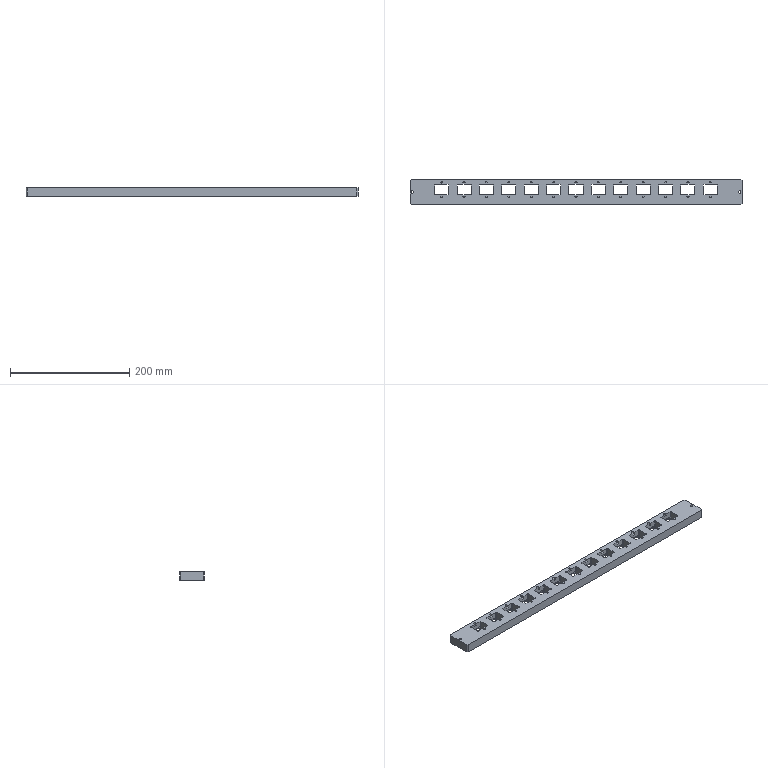NC program | NX | posted with a generic post | part box 556 x 41 x 15 mm
Lines 1 to 872 of 52182:
N10 G17 G21 G94 G90
(ZLEVEL_PROFILE_COPY_1_COPY_COPY_3 , TOOL : D6JING)
N12 T06 M6
N14 G54
N16 G17 G0 G90 X220.712 Y-3.45 S5000 M3
N18 G43 Z30. H6
N20 Z-0.147
N22 G94 G1 X219.631 Y-4.121 F1000.
N24 G3 X219.348 Y-4.65 R0.6
N26 G1 X230.652 F1800.
N28 G3 X230.369 Y-4.121 R0.6
N30 G1 X229.288 Y-3.45
N32 G0 X220.712 Z-0.294
N34 G1 X219.631 Y-4.121 F1000.
N36 G3 X219.348 Y-4.65 R0.6
N38 G1 X230.652 F1800.
N40 G3 X230.369 Y-4.121 R0.6
N42 G1 X229.288 Y-3.45
N44 G0 X220.712 Z-0.441
N46 G1 X219.631 Y-4.121 F1000.
N48 G3 X219.348 Y-4.65 R0.6
N50 G1 X230.652 F1800.
N52 G3 X230.369 Y-4.121 R0.6
N54 G1 X229.288 Y-3.45
N56 G0 X220.712 Z-0.588
N58 G1 X219.631 Y-4.121 F1000.
N60 G3 X219.348 Y-4.65 R0.6
N62 G1 X230.652 F1800.
N64 G3 X230.369 Y-4.121 R0.6
N66 G1 X229.288 Y-3.45
N68 G0 X220.712 Z-0.735
N70 G1 X219.631 Y-4.121 F1000.
N72 G3 X219.348 Y-4.65 R0.6
N74 G1 X230.652 F1800.
N76 G3 X230.369 Y-4.121 R0.6
N78 G1 X229.288 Y-3.45
N80 G0 X220.712 Z-0.882
N82 G1 X219.631 Y-4.121 F1000.
N84 G3 X219.348 Y-4.65 R0.6
N86 G1 X230.652 F1800.
N88 G3 X230.369 Y-4.121 R0.6
N90 G1 X229.288 Y-3.45
N92 G0 X220.712 Z-1.029
N94 G1 X219.631 Y-4.121 F1000.
N96 G3 X219.348 Y-4.65 R0.6
N98 G1 X230.652 F1800.
N100 G3 X230.369 Y-4.121 R0.6
N102 G1 X229.288 Y-3.45
N104 G0 X220.712 Z-1.176
N106 G1 X219.631 Y-4.121 F1000.
N108 G3 X219.348 Y-4.65 R0.6
N110 G1 X230.652 F1800.
N112 G3 X230.369 Y-4.121 R0.6
N114 G1 X229.288 Y-3.45
N116 G0 X220.712 Z-1.324
N118 G1 X219.631 Y-4.121 F1000.
N120 G3 X219.348 Y-4.65 R0.6
N122 G1 X230.652 F1800.
N124 G3 X230.369 Y-4.121 R0.6
N126 G1 X229.288 Y-3.45
N128 G0 X220.712 Z-1.471
N130 G1 X219.631 Y-4.121 F1000.
N132 G3 X219.348 Y-4.65 R0.6
N134 G1 X230.652 F1800.
N136 G3 X230.369 Y-4.121 R0.6
N138 G1 X229.288 Y-3.45
N140 G0 X220.712 Z-1.618
N142 G1 X219.631 Y-4.121 F1000.
N144 G3 X219.348 Y-4.65 R0.6
N146 G1 X230.652 F1800.
N148 G3 X230.369 Y-4.121 R0.6
N150 G1 X229.288 Y-3.45
N152 G0 X220.712 Z-1.765
N154 G1 X219.631 Y-4.121 F1000.
N156 G3 X219.348 Y-4.65 R0.6
N158 G1 X230.652 F1800.
N160 G3 X230.369 Y-4.121 R0.6
N162 G1 X229.288 Y-3.45
N164 G0 X220.712 Z-1.912
N166 G1 X219.631 Y-4.121 F1000.
N168 G3 X219.348 Y-4.65 R0.6
N170 G1 X230.652 F1800.
N172 G3 X230.369 Y-4.121 R0.6
N174 G1 X229.288 Y-3.45
N176 G0 X220.712 Z-2.059
N178 G1 X219.631 Y-4.121 F1000.
N180 G3 X219.348 Y-4.65 R0.6
N182 G1 X230.652 F1800.
N184 G3 X230.369 Y-4.121 R0.6
N186 G1 X229.288 Y-3.45
N188 G0 X220.712 Z-2.206
N190 G1 X219.631 Y-4.121 F1000.
N192 G3 X219.348 Y-4.65 R0.6
N194 G1 X230.652 F1800.
N196 G3 X230.369 Y-4.121 R0.6
N198 G1 X229.288 Y-3.45
N200 G0 X220.712 Z-2.353
N202 G1 X219.631 Y-4.121 F1000.
N204 G3 X219.348 Y-4.65 R0.6
N206 G1 X230.652 F1800.
N208 G3 X230.369 Y-4.121 R0.6
N210 G1 X229.288 Y-3.45
N212 G0 X220.712 Z-2.5
N214 G1 X219.631 Y-4.121 F1000.
N216 G3 X219.348 Y-4.65 R0.6
N218 G1 X230.652 F1800.
N220 G3 X230.369 Y-4.121 R0.6
N222 G1 X229.288 Y-3.45
N224 G0 X220.712 Z-2.647
N226 G1 X219.631 Y-4.121 F1000.
N228 G3 X219.348 Y-4.65 R0.6
N230 G1 X230.652 F1800.
N232 G3 X230.369 Y-4.121 R0.6
N234 G1 X229.288 Y-3.45
N236 G0 X220.712 Z-2.794
N238 G1 X219.631 Y-4.121 F1000.
N240 G3 X219.348 Y-4.65 R0.6
N242 G1 X230.652 F1800.
N244 G3 X230.369 Y-4.121 R0.6
N246 G1 X229.288 Y-3.45
N248 G0 X220.712 Z-2.941
N250 G1 X219.631 Y-4.121 F1000.
N252 G3 X219.348 Y-4.65 R0.6
N254 G1 X230.652 F1800.
N256 G3 X230.369 Y-4.121 R0.6
N258 G1 X229.288 Y-3.45
N260 G0 X220.712 Z-3.088
N262 G1 X219.631 Y-4.121 F1000.
N264 G3 X219.348 Y-4.65 R0.6
N266 G1 X230.652 F1800.
N268 G3 X230.369 Y-4.121 R0.6
N270 G1 X229.288 Y-3.45
N272 G0 X220.712 Z-3.235
N274 G1 X219.631 Y-4.121 F1000.
N276 G3 X219.348 Y-4.65 R0.6
N278 G1 X230.652 F1800.
N280 G3 X230.369 Y-4.121 R0.6
N282 G1 X229.288 Y-3.45
N284 G0 X220.712 Z-3.382
N286 G1 X219.631 Y-4.121 F1000.
N288 G3 X219.348 Y-4.65 R0.6
N290 G1 X230.652 F1800.
N292 G3 X230.369 Y-4.121 R0.6
N294 G1 X229.288 Y-3.45
N296 G0 X220.712 Z-3.529
N298 G1 X219.631 Y-4.121 F1000.
N300 G3 X219.348 Y-4.65 R0.6
N302 G1 X230.652 F1800.
N304 G3 X230.369 Y-4.121 R0.6
N306 G1 X229.288 Y-3.45
N308 G0 X220.712 Z-3.676
N310 G1 X219.631 Y-4.121 F1000.
N312 G3 X219.348 Y-4.65 R0.6
N314 G1 X230.652 F1800.
N316 G3 X230.369 Y-4.121 R0.6
N318 G1 X229.288 Y-3.45
N320 G0 X220.712 Z-3.824
N322 G1 X219.631 Y-4.121 F1000.
N324 G3 X219.348 Y-4.65 R0.6
N326 G1 X230.652 F1800.
N328 G3 X230.369 Y-4.121 R0.6
N330 G1 X229.288 Y-3.45
N332 G0 X220.712 Z-3.971
N334 G1 X219.631 Y-4.121 F1000.
N336 G3 X219.348 Y-4.65 R0.6
N338 G1 X230.652 F1800.
N340 G3 X230.369 Y-4.121 R0.6
N342 G1 X229.288 Y-3.45
N344 G0 X220.712 Z-4.118
N346 G1 X219.631 Y-4.121 F1000.
N348 G3 X219.348 Y-4.65 R0.6
N350 G1 X230.652 F1800.
N352 G3 X230.369 Y-4.121 R0.6
N354 G1 X229.288 Y-3.45
N356 G0 X220.712 Z-4.265
N358 G1 X219.631 Y-4.121 F1000.
N360 G3 X219.348 Y-4.65 R0.6
N362 G1 X230.652 F1800.
N364 G3 X230.369 Y-4.121 R0.6
N366 G1 X229.288 Y-3.45
N368 G0 X220.712 Z-4.412
N370 G1 X219.631 Y-4.121 F1000.
N372 G3 X219.348 Y-4.65 R0.6
N374 G1 X230.652 F1800.
N376 G3 X230.369 Y-4.121 R0.6
N378 G1 X229.288 Y-3.45
N380 G0 X220.712 Z-4.559
N382 G1 X219.631 Y-4.121 F1000.
N384 G3 X219.348 Y-4.65 R0.6
N386 G1 X230.652 F1800.
N388 G3 X230.369 Y-4.121 R0.6
N390 G1 X229.288 Y-3.45
N392 G0 X220.712 Z-4.706
N394 G1 X219.631 Y-4.121 F1000.
N396 G3 X219.348 Y-4.65 R0.6
N398 G1 X230.652 F1800.
N400 G3 X230.369 Y-4.121 R0.6
N402 G1 X229.288 Y-3.45
N404 G0 X220.712 Z-4.853
N406 G1 X219.631 Y-4.121 F1000.
N408 G3 X219.348 Y-4.65 R0.6
N410 G1 X230.652 F1800.
N412 G3 X230.369 Y-4.121 R0.6
N414 G1 X229.288 Y-3.45
N416 G0 X220.712 Z-5.
N418 G1 X219.631 Y-4.121 F1000.
N420 G3 X219.348 Y-4.65 R0.6
N422 G1 X230.652 F1800.
N424 G3 X230.369 Y-4.121 R0.6
N426 G1 X229.288 Y-3.45
N428 G0 Z30.
N430 Y11.45
N432 Z-0.147
N434 G1 X230.369 Y12.121 F1000.
N436 G3 X230.652 Y12.65 R0.6
N438 G1 X219.348 F1800.
N440 G3 X219.631 Y12.121 R0.6
N442 G1 X220.712 Y11.45
N444 G0 X229.288 Z-0.294
N446 G1 X230.369 Y12.121 F1000.
N448 G3 X230.652 Y12.65 R0.6
N450 G1 X219.348 F1800.
N452 G3 X219.631 Y12.121 R0.6
N454 G1 X220.712 Y11.45
N456 G0 X229.288 Z-0.441
N458 G1 X230.369 Y12.121 F1000.
N460 G3 X230.652 Y12.65 R0.6
N462 G1 X219.348 F1800.
N464 G3 X219.631 Y12.121 R0.6
N466 G1 X220.712 Y11.45
N468 G0 X229.288 Z-0.588
N470 G1 X230.369 Y12.121 F1000.
N472 G3 X230.652 Y12.65 R0.6
N474 G1 X219.348 F1800.
N476 G3 X219.631 Y12.121 R0.6
N478 G1 X220.712 Y11.45
N480 G0 X229.288 Z-0.735
N482 G1 X230.369 Y12.121 F1000.
N484 G3 X230.652 Y12.65 R0.6
N486 G1 X219.348 F1800.
N488 G3 X219.631 Y12.121 R0.6
N490 G1 X220.712 Y11.45
N492 G0 X229.288 Z-0.882
N494 G1 X230.369 Y12.121 F1000.
N496 G3 X230.652 Y12.65 R0.6
N498 G1 X219.348 F1800.
N500 G3 X219.631 Y12.121 R0.6
N502 G1 X220.712 Y11.45
N504 G0 X229.288 Z-1.029
N506 G1 X230.369 Y12.121 F1000.
N508 G3 X230.652 Y12.65 R0.6
N510 G1 X219.348 F1800.
N512 G3 X219.631 Y12.121 R0.6
N514 G1 X220.712 Y11.45
N516 G0 X229.288 Z-1.176
N518 G1 X230.369 Y12.121 F1000.
N520 G3 X230.652 Y12.65 R0.6
N522 G1 X219.348 F1800.
N524 G3 X219.631 Y12.121 R0.6
N526 G1 X220.712 Y11.45
N528 G0 X229.288 Z-1.324
N530 G1 X230.369 Y12.121 F1000.
N532 G3 X230.652 Y12.65 R0.6
N534 G1 X219.348 F1800.
N536 G3 X219.631 Y12.121 R0.6
N538 G1 X220.712 Y11.45
N540 G0 X229.288 Z-1.471
N542 G1 X230.369 Y12.121 F1000.
N544 G3 X230.652 Y12.65 R0.6
N546 G1 X219.348 F1800.
N548 G3 X219.631 Y12.121 R0.6
N550 G1 X220.712 Y11.45
N552 G0 X229.288 Z-1.618
N554 G1 X230.369 Y12.121 F1000.
N556 G3 X230.652 Y12.65 R0.6
N558 G1 X219.348 F1800.
N560 G3 X219.631 Y12.121 R0.6
N562 G1 X220.712 Y11.45
N564 G0 X229.288 Z-1.765
N566 G1 X230.369 Y12.121 F1000.
N568 G3 X230.652 Y12.65 R0.6
N570 G1 X219.348 F1800.
N572 G3 X219.631 Y12.121 R0.6
N574 G1 X220.712 Y11.45
N576 G0 X229.288 Z-1.912
N578 G1 X230.369 Y12.121 F1000.
N580 G3 X230.652 Y12.65 R0.6
N582 G1 X219.348 F1800.
N584 G3 X219.631 Y12.121 R0.6
N586 G1 X220.712 Y11.45
N588 G0 X229.288 Z-2.059
N590 G1 X230.369 Y12.121 F1000.
N592 G3 X230.652 Y12.65 R0.6
N594 G1 X219.348 F1800.
N596 G3 X219.631 Y12.121 R0.6
N598 G1 X220.712 Y11.45
N600 G0 X229.288 Z-2.206
N602 G1 X230.369 Y12.121 F1000.
N604 G3 X230.652 Y12.65 R0.6
N606 G1 X219.348 F1800.
N608 G3 X219.631 Y12.121 R0.6
N610 G1 X220.712 Y11.45
N612 G0 X229.288 Z-2.353
N614 G1 X230.369 Y12.121 F1000.
N616 G3 X230.652 Y12.65 R0.6
N618 G1 X219.348 F1800.
N620 G3 X219.631 Y12.121 R0.6
N622 G1 X220.712 Y11.45
N624 G0 X229.288 Z-2.5
N626 G1 X230.369 Y12.121 F1000.
N628 G3 X230.652 Y12.65 R0.6
N630 G1 X219.348 F1800.
N632 G3 X219.631 Y12.121 R0.6
N634 G1 X220.712 Y11.45
N636 G0 X229.288 Z-2.647
N638 G1 X230.369 Y12.121 F1000.
N640 G3 X230.652 Y12.65 R0.6
N642 G1 X219.348 F1800.
N644 G3 X219.631 Y12.121 R0.6
N646 G1 X220.712 Y11.45
N648 G0 X229.288 Z-2.794
N650 G1 X230.369 Y12.121 F1000.
N652 G3 X230.652 Y12.65 R0.6
N654 G1 X219.348 F1800.
N656 G3 X219.631 Y12.121 R0.6
N658 G1 X220.712 Y11.45
N660 G0 X229.288 Z-2.941
N662 G1 X230.369 Y12.121 F1000.
N664 G3 X230.652 Y12.65 R0.6
N666 G1 X219.348 F1800.
N668 G3 X219.631 Y12.121 R0.6
N670 G1 X220.712 Y11.45
N672 G0 X229.288 Z-3.088
N674 G1 X230.369 Y12.121 F1000.
N676 G3 X230.652 Y12.65 R0.6
N678 G1 X219.348 F1800.
N680 G3 X219.631 Y12.121 R0.6
N682 G1 X220.712 Y11.45
N684 G0 X229.288 Z-3.235
N686 G1 X230.369 Y12.121 F1000.
N688 G3 X230.652 Y12.65 R0.6
N690 G1 X219.348 F1800.
N692 G3 X219.631 Y12.121 R0.6
N694 G1 X220.712 Y11.45
N696 G0 X229.288 Z-3.382
N698 G1 X230.369 Y12.121 F1000.
N700 G3 X230.652 Y12.65 R0.6
N702 G1 X219.348 F1800.
N704 G3 X219.631 Y12.121 R0.6
N706 G1 X220.712 Y11.45
N708 G0 X229.288 Z-3.529
N710 G1 X230.369 Y12.121 F1000.
N712 G3 X230.652 Y12.65 R0.6
N714 G1 X219.348 F1800.
N716 G3 X219.631 Y12.121 R0.6
N718 G1 X220.712 Y11.45
N720 G0 X229.288 Z-3.676
N722 G1 X230.369 Y12.121 F1000.
N724 G3 X230.652 Y12.65 R0.6
N726 G1 X219.348 F1800.
N728 G3 X219.631 Y12.121 R0.6
N730 G1 X220.712 Y11.45
N732 G0 X229.288 Z-3.824
N734 G1 X230.369 Y12.121 F1000.
N736 G3 X230.652 Y12.65 R0.6
N738 G1 X219.348 F1800.
N740 G3 X219.631 Y12.121 R0.6
N742 G1 X220.712 Y11.45
N744 G0 X229.288 Z-3.971
N746 G1 X230.369 Y12.121 F1000.
N748 G3 X230.652 Y12.65 R0.6
N750 G1 X219.348 F1800.
N752 G3 X219.631 Y12.121 R0.6
N754 G1 X220.712 Y11.45
N756 G0 X229.288 Z-4.118
N758 G1 X230.369 Y12.121 F1000.
N760 G3 X230.652 Y12.65 R0.6
N762 G1 X219.348 F1800.
N764 G3 X219.631 Y12.121 R0.6
N766 G1 X220.712 Y11.45
N768 G0 X229.288 Z-4.265
N770 G1 X230.369 Y12.121 F1000.
N772 G3 X230.652 Y12.65 R0.6
N774 G1 X219.348 F1800.
N776 G3 X219.631 Y12.121 R0.6
N778 G1 X220.712 Y11.45
N780 G0 X229.288 Z-4.412
N782 G1 X230.369 Y12.121 F1000.
N784 G3 X230.652 Y12.65 R0.6
N786 G1 X219.348 F1800.
N788 G3 X219.631 Y12.121 R0.6
N790 G1 X220.712 Y11.45
N792 G0 X229.288 Z-4.559
N794 G1 X230.369 Y12.121 F1000.
N796 G3 X230.652 Y12.65 R0.6
N798 G1 X219.348 F1800.
N800 G3 X219.631 Y12.121 R0.6
N802 G1 X220.712 Y11.45
N804 G0 X229.288 Z-4.706
N806 G1 X230.369 Y12.121 F1000.
N808 G3 X230.652 Y12.65 R0.6
N810 G1 X219.348 F1800.
N812 G3 X219.631 Y12.121 R0.6
N814 G1 X220.712 Y11.45
N816 G0 X229.288 Z-4.853
N818 G1 X230.369 Y12.121 F1000.
N820 G3 X230.652 Y12.65 R0.6
N822 G1 X219.348 F1800.
N824 G3 X219.631 Y12.121 R0.6
N826 G1 X220.712 Y11.45
N828 G0 X229.288 Z-5.
N830 G1 X230.369 Y12.121 F1000.
N832 G3 X230.652 Y12.65 R0.6
N834 G1 X219.348 F1800.
N836 G3 X219.631 Y12.121 R0.6
N838 G1 X220.712 Y11.45
N840 G0 Z30.
N842 X183.212 Y-3.45
N844 Z-0.147
N846 G1 X182.131 Y-4.121 F1000.
N848 G3 X181.848 Y-4.65 R0.6
N850 G1 X193.152 F1800.
N852 G3 X192.869 Y-4.121 R0.6
N854 G1 X191.788 Y-3.45
N856 G0 X183.212 Z-0.294
N858 G1 X182.131 Y-4.121 F1000.
N860 G3 X181.848 Y-4.65 R0.6
N862 G1 X193.152 F1800.
N864 G3 X192.869 Y-4.121 R0.6
N866 G1 X191.788 Y-3.45
N868 G0 X183.212 Z-0.441
N870 G1 X182.131 Y-4.121 F1000.
N872 G3 X181.848 Y-4.65 R0.6
N874 G1 X193.152 F1800.
N876 G3 X192.869 Y-4.121 R0.6
N878 G1 X191.788 Y-3.45
N880 G0 X183.212 Z-0.588
N882 G1 X182.131 Y-4.121 F1000.
N884 G3 X181.848 Y-4.65 R0.6
N886 G1 X193.152 F1800.
N888 G3 X192.869 Y-4.121 R0.6
N890 G1 X191.788 Y-3.45
N892 G0 X183.212 Z-0.735
N894 G1 X182.131 Y-4.121 F1000.
N896 G3 X181.848 Y-4.65 R0.6
N898 G1 X193.152 F1800.
N900 G3 X192.869 Y-4.121 R0.6
N902 G1 X191.788 Y-3.45
N904 G0 X183.212 Z-0.882
N906 G1 X182.131 Y-4.121 F1000.
N908 G3 X181.848 Y-4.65 R0.6
N910 G1 X193.152 F1800.
N912 G3 X192.869 Y-4.121 R0.6
N914 G1 X191.788 Y-3.45
N916 G0 X183.212 Z-1.029
N918 G1 X182.131 Y-4.121 F1000.
N920 G3 X181.848 Y-4.65 R0.6
N922 G1 X193.152 F1800.
N924 G3 X192.869 Y-4.121 R0.6
N926 G1 X191.788 Y-3.45
N928 G0 X183.212 Z-1.176
N930 G1 X182.131 Y-4.121 F1000.
N932 G3 X181.848 Y-4.65 R0.6
N934 G1 X193.152 F1800.
N936 G3 X192.869 Y-4.121 R0.6
N938 G1 X191.788 Y-3.45
N940 G0 X183.212 Z-1.324
N942 G1 X182.131 Y-4.121 F1000.
N944 G3 X181.848 Y-4.65 R0.6
N946 G1 X193.152 F1800.
N948 G3 X192.869 Y-4.121 R0.6
N950 G1 X191.788 Y-3.45
N952 G0 X183.212 Z-1.471
N954 G1 X182.131 Y-4.121 F1000.
N956 G3 X181.848 Y-4.65 R0.6
N958 G1 X193.152 F1800.
N960 G3 X192.869 Y-4.121 R0.6
N962 G1 X191.788 Y-3.45
N964 G0 X183.212 Z-1.618
N966 G1 X182.131 Y-4.121 F1000.
N968 G3 X181.848 Y-4.65 R0.6
N970 G1 X193.152 F1800.
N972 G3 X192.869 Y-4.121 R0.6
N974 G1 X191.788 Y-3.45
N976 G0 X183.212 Z-1.765
N978 G1 X182.131 Y-4.121 F1000.
N980 G3 X181.848 Y-4.65 R0.6
N982 G1 X193.152 F1800.
N984 G3 X192.869 Y-4.121 R0.6
N986 G1 X191.788 Y-3.45
N988 G0 X183.212 Z-1.912
N990 G1 X182.131 Y-4.121 F1000.
N992 G3 X181.848 Y-4.65 R0.6
N994 G1 X193.152 F1800.
N996 G3 X192.869 Y-4.121 R0.6
N998 G1 X191.788 Y-3.45
N1000 G0 X183.212 Z-2.059
N1002 G1 X182.131 Y-4.121 F1000.
N1004 G3 X181.848 Y-4.65 R0.6
N1006 G1 X193.152 F1800.
N1008 G3 X192.869 Y-4.121 R0.6
N1010 G1 X191.788 Y-3.45
N1012 G0 X183.212 Z-2.206
N1014 G1 X182.131 Y-4.121 F1000.
N1016 G3 X181.848 Y-4.65 R0.6
N1018 G1 X193.152 F1800.
N1020 G3 X192.869 Y-4.121 R0.6
N1022 G1 X191.788 Y-3.45
N1024 G0 X183.212 Z-2.353
N1026 G1 X182.131 Y-4.121 F1000.
N1028 G3 X181.848 Y-4.65 R0.6
N1030 G1 X193.152 F1800.
N1032 G3 X192.869 Y-4.121 R0.6
N1034 G1 X191.788 Y-3.45
N1036 G0 X183.212 Z-2.5
N1038 G1 X182.131 Y-4.121 F1000.
N1040 G3 X181.848 Y-4.65 R0.6
N1042 G1 X193.152 F1800.
N1044 G3 X192.869 Y-4.121 R0.6
N1046 G1 X191.788 Y-3.45
N1048 G0 X183.212 Z-2.647
N1050 G1 X182.131 Y-4.121 F1000.
N1052 G3 X181.848 Y-4.65 R0.6
N1054 G1 X193.152 F1800.
N1056 G3 X192.869 Y-4.121 R0.6
N1058 G1 X191.788 Y-3.45
N1060 G0 X183.212 Z-2.794
N1062 G1 X182.131 Y-4.121 F1000.
N1064 G3 X181.848 Y-4.65 R0.6
N1066 G1 X193.152 F1800.
N1068 G3 X192.869 Y-4.121 R0.6
N1070 G1 X191.788 Y-3.45
N1072 G0 X183.212 Z-2.941
N1074 G1 X182.131 Y-4.121 F1000.
N1076 G3 X181.848 Y-4.65 R0.6
N1078 G1 X193.152 F1800.
N1080 G3 X192.869 Y-4.121 R0.6
N1082 G1 X191.788 Y-3.45
N1084 G0 X183.212 Z-3.088
N1086 G1 X182.131 Y-4.121 F1000.
N1088 G3 X181.848 Y-4.65 R0.6
N1090 G1 X193.152 F1800.
N1092 G3 X192.869 Y-4.121 R0.6
N1094 G1 X191.788 Y-3.45
N1096 G0 X183.212 Z-3.235
N1098 G1 X182.131 Y-4.121 F1000.
N1100 G3 X181.848 Y-4.65 R0.6
N1102 G1 X193.152 F1800.
N1104 G3 X192.869 Y-4.121 R0.6
N1106 G1 X191.788 Y-3.45
N1108 G0 X183.212 Z-3.382
N1110 G1 X182.131 Y-4.121 F1000.
N1112 G3 X181.848 Y-4.65 R0.6
N1114 G1 X193.152 F1800.
N1116 G3 X192.869 Y-4.121 R0.6
N1118 G1 X191.788 Y-3.45
N1120 G0 X183.212 Z-3.529
N1122 G1 X182.131 Y-4.121 F1000.
N1124 G3 X181.848 Y-4.65 R0.6
N1126 G1 X193.152 F1800.
N1128 G3 X192.869 Y-4.121 R0.6
N1130 G1 X191.788 Y-3.45
N1132 G0 X183.212 Z-3.676
N1134 G1 X182.131 Y-4.121 F1000.
N1136 G3 X181.848 Y-4.65 R0.6
N1138 G1 X193.152 F1800.
N1140 G3 X192.869 Y-4.121 R0.6
N1142 G1 X191.788 Y-3.45
N1144 G0 X183.212 Z-3.824
N1146 G1 X182.131 Y-4.121 F1000.
N1148 G3 X181.848 Y-4.65 R0.6
N1150 G1 X193.152 F1800.
N1152 G3 X192.869 Y-4.121 R0.6
N1154 G1 X191.788 Y-3.45
N1156 G0 X183.212 Z-3.971
N1158 G1 X182.131 Y-4.121 F1000.
N1160 G3 X181.848 Y-4.65 R0.6
N1162 G1 X193.152 F1800.
N1164 G3 X192.869 Y-4.121 R0.6
N1166 G1 X191.788 Y-3.45
N1168 G0 X183.212 Z-4.118
N1170 G1 X182.131 Y-4.121 F1000.
N1172 G3 X181.848 Y-4.65 R0.6
N1174 G1 X193.152 F1800.
N1176 G3 X192.869 Y-4.121 R0.6
N1178 G1 X191.788 Y-3.45
N1180 G0 X183.212 Z-4.265
N1182 G1 X182.131 Y-4.121 F1000.
N1184 G3 X181.848 Y-4.65 R0.6
N1186 G1 X193.152 F1800.
N1188 G3 X192.869 Y-4.121 R0.6
N1190 G1 X191.788 Y-3.45
N1192 G0 X183.212 Z-4.412
N1194 G1 X182.131 Y-4.121 F1000.
N1196 G3 X181.848 Y-4.65 R0.6
N1198 G1 X193.152 F1800.
N1200 G3 X192.869 Y-4.121 R0.6
N1202 G1 X191.788 Y-3.45
N1204 G0 X183.212 Z-4.559
N1206 G1 X182.131 Y-4.121 F1000.
N1208 G3 X181.848 Y-4.65 R0.6
N1210 G1 X193.152 F1800.
N1212 G3 X192.869 Y-4.121 R0.6
N1214 G1 X191.788 Y-3.45
N1216 G0 X183.212 Z-4.706
N1218 G1 X182.131 Y-4.121 F1000.
N1220 G3 X181.848 Y-4.65 R0.6
N1222 G1 X193.152 F1800.
N1224 G3 X192.869 Y-4.121 R0.6
N1226 G1 X191.788 Y-3.45
N1228 G0 X183.212 Z-4.853
N1230 G1 X182.131 Y-4.121 F1000.
N1232 G3 X181.848 Y-4.65 R0.6
N1234 G1 X193.152 F1800.
N1236 G3 X192.869 Y-4.121 R0.6
N1238 G1 X191.788 Y-3.45
N1240 G0 X183.212 Z-5.
N1242 G1 X182.131 Y-4.121 F1000.
N1244 G3 X181.848 Y-4.65 R0.6
N1246 G1 X193.152 F1800.
N1248 G3 X192.869 Y-4.121 R0.6
N1250 G1 X191.788 Y-3.45
N1252 G0 Z30.
N1254 Y11.45
N1256 Z-0.147
N1258 G1 X192.869 Y12.121 F1000.
N1260 G3 X193.152 Y12.65 R0.6
N1262 G1 X181.848 F1800.
N1264 G3 X182.131 Y12.121 R0.6
N1266 G1 X183.212 Y11.45
N1268 G0 X191.788 Z-0.294
N1270 G1 X192.869 Y12.121 F1000.
N1272 G3 X193.152 Y12.65 R0.6
N1274 G1 X181.848 F1800.
N1276 G3 X182.131 Y12.121 R0.6
N1278 G1 X183.212 Y11.45
N1280 G0 X191.788 Z-0.441
N1282 G1 X192.869 Y12.121 F1000.
N1284 G3 X193.152 Y12.65 R0.6
N1286 G1 X181.848 F1800.
N1288 G3 X182.131 Y12.121 R0.6
N1290 G1 X183.212 Y11.45
N1292 G0 X191.788 Z-0.588
N1294 G1 X192.869 Y12.121 F1000.
N1296 G3 X193.152 Y12.65 R0.6
N1298 G1 X181.848 F1800.
N1300 G3 X182.131 Y12.121 R0.6
N1302 G1 X183.212 Y11.45
N1304 G0 X191.788 Z-0.735
N1306 G1 X192.869 Y12.121 F1000.
N1308 G3 X193.152 Y12.65 R0.6
N1310 G1 X181.848 F1800.
N1312 G3 X182.131 Y12.121 R0.6
N1314 G1 X183.212 Y11.45
N1316 G0 X191.788 Z-0.882
N1318 G1 X192.869 Y12.121 F1000.
N1320 G3 X193.152 Y12.65 R0.6
N1322 G1 X181.848 F1800.
N1324 G3 X182.131 Y12.121 R0.6
N1326 G1 X183.212 Y11.45
N1328 G0 X191.788 Z-1.029
N1330 G1 X192.869 Y12.121 F1000.
N1332 G3 X193.152 Y12.65 R0.6
N1334 G1 X181.848 F1800.
N1336 G3 X182.131 Y12.121 R0.6
N1338 G1 X183.212 Y11.45
N1340 G0 X191.788 Z-1.176
N1342 G1 X192.869 Y12.121 F1000.
N1344 G3 X193.152 Y12.65 R0.6
N1346 G1 X181.848 F1800.
N1348 G3 X182.131 Y12.121 R0.6
N1350 G1 X183.212 Y11.45
N1352 G0 X191.788 Z-1.324
N1354 G1 X192.869 Y12.121 F1000.
N1356 G3 X193.152 Y12.65 R0.6
N1358 G1 X181.848 F1800.
N1360 G3 X182.131 Y12.121 R0.6
N1362 G1 X183.212 Y11.45
N1364 G0 X191.788 Z-1.471
N1366 G1 X192.869 Y12.121 F1000.
N1368 G3 X193.152 Y12.65 R0.6
N1370 G1 X181.848 F1800.
N1372 G3 X182.131 Y12.121 R0.6
N1374 G1 X183.212 Y11.45
N1376 G0 X191.788 Z-1.618
N1378 G1 X192.869 Y12.121 F1000.
N1380 G3 X193.152 Y12.65 R0.6
N1382 G1 X181.848 F1800.
N1384 G3 X182.131 Y12.121 R0.6
N1386 G1 X183.212 Y11.45
N1388 G0 X191.788 Z-1.765
N1390 G1 X192.869 Y12.121 F1000.
N1392 G3 X193.152 Y12.65 R0.6
N1394 G1 X181.848 F1800.
N1396 G3 X182.131 Y12.121 R0.6
N1398 G1 X183.212 Y11.45
N1400 G0 X191.788 Z-1.912
N1402 G1 X192.869 Y12.121 F1000.
N1404 G3 X193.152 Y12.65 R0.6
N1406 G1 X181.848 F1800.
N1408 G3 X182.131 Y12.121 R0.6
N1410 G1 X183.212 Y11.45
N1412 G0 X191.788 Z-2.059
N1414 G1 X192.869 Y12.121 F1000.
N1416 G3 X193.152 Y12.65 R0.6
N1418 G1 X181.848 F1800.
N1420 G3 X182.131 Y12.121 R0.6
N1422 G1 X183.212 Y11.45
N1424 G0 X191.788 Z-2.206
N1426 G1 X192.869 Y12.121 F1000.
N1428 G3 X193.152 Y12.65 R0.6
N1430 G1 X181.848 F1800.
N1432 G3 X182.131 Y12.121 R0.6
N1434 G1 X183.212 Y11.45
N1436 G0 X191.788 Z-2.353
N1438 G1 X192.869 Y12.121 F1000.
N1440 G3 X193.152 Y12.65 R0.6
N1442 G1 X181.848 F1800.
N1444 G3 X182.131 Y12.121 R0.6
N1446 G1 X183.212 Y11.45
N1448 G0 X191.788 Z-2.5
N1450 G1 X192.869 Y12.121 F1000.
N1452 G3 X193.152 Y12.65 R0.6
N1454 G1 X181.848 F1800.
N1456 G3 X182.131 Y12.121 R0.6
N1458 G1 X183.212 Y11.45
N1460 G0 X191.788 Z-2.647
N1462 G1 X192.869 Y12.121 F1000.
N1464 G3 X193.152 Y12.65 R0.6
N1466 G1 X181.848 F1800.
N1468 G3 X182.131 Y12.121 R0.6
N1470 G1 X183.212 Y11.45
N1472 G0 X191.788 Z-2.794
N1474 G1 X192.869 Y12.121 F1000.
N1476 G3 X193.152 Y12.65 R0.6
N1478 G1 X181.848 F1800.
N1480 G3 X182.131 Y12.121 R0.6
N1482 G1 X183.212 Y11.45
N1484 G0 X191.788 Z-2.941
N1486 G1 X192.869 Y12.121 F1000.
N1488 G3 X193.152 Y12.65 R0.6
N1490 G1 X181.848 F1800.
N1492 G3 X182.131 Y12.121 R0.6
N1494 G1 X183.212 Y11.45
N1496 G0 X191.788 Z-3.088
N1498 G1 X192.869 Y12.121 F1000.
N1500 G3 X193.152 Y12.65 R0.6
N1502 G1 X181.848 F1800.
N1504 G3 X182.131 Y12.121 R0.6
N1506 G1 X183.212 Y11.45
N1508 G0 X191.788 Z-3.235
N1510 G1 X192.869 Y12.121 F1000.
N1512 G3 X193.152 Y12.65 R0.6
N1514 G1 X181.848 F1800.
N1516 G3 X182.131 Y12.121 R0.6
N1518 G1 X183.212 Y11.45
N1520 G0 X191.788 Z-3.382
N1522 G1 X192.869 Y12.121 F1000.
N1524 G3 X193.152 Y12.65 R0.6
N1526 G1 X181.848 F1800.
N1528 G3 X182.131 Y12.121 R0.6
N1530 G1 X183.212 Y11.45
N1532 G0 X191.788 Z-3.529
N1534 G1 X192.869 Y12.121 F1000.
N1536 G3 X193.152 Y12.65 R0.6
N1538 G1 X181.848 F1800.
N1540 G3 X182.131 Y12.121 R0.6
N1542 G1 X183.212 Y11.45
N1544 G0 X191.788 Z-3.676
N1546 G1 X192.869 Y12.121 F1000.
N1548 G3 X193.152 Y12.65 R0.6
N1550 G1 X181.848 F1800.
N1552 G3 X182.131 Y12.121 R0.6
N1554 G1 X183.212 Y11.45
N1556 G0 X191.788 Z-3.824
N1558 G1 X192.869 Y12.121 F1000.
N1560 G3 X193.152 Y12.65 R0.6
N1562 G1 X181.848 F1800.
N1564 G3 X182.131 Y12.121 R0.6
N1566 G1 X183.212 Y11.45
N1568 G0 X191.788 Z-3.971
N1570 G1 X192.869 Y12.121 F1000.
N1572 G3 X193.152 Y12.65 R0.6
N1574 G1 X181.848 F1800.
N1576 G3 X182.131 Y12.121 R0.6
N1578 G1 X183.212 Y11.45
N1580 G0 X191.788 Z-4.118
N1582 G1 X192.869 Y12.121 F1000.
N1584 G3 X193.152 Y12.65 R0.6
N1586 G1 X181.848 F1800.
N1588 G3 X182.131 Y12.121 R0.6
N1590 G1 X183.212 Y11.45
N1592 G0 X191.788 Z-4.265
N1594 G1 X192.869 Y12.121 F1000.
N1596 G3 X193.152 Y12.65 R0.6
N1598 G1 X181.848 F1800.
N1600 G3 X182.131 Y12.121 R0.6
N1602 G1 X183.212 Y11.45
N1604 G0 X191.788 Z-4.412
N1606 G1 X192.869 Y12.121 F1000.
N1608 G3 X193.152 Y12.65 R0.6
N1610 G1 X181.848 F1800.
N1612 G3 X182.131 Y12.121 R0.6
N1614 G1 X183.212 Y11.45
N1616 G0 X191.788 Z-4.559
N1618 G1 X192.869 Y12.121 F1000.
N1620 G3 X193.152 Y12.65 R0.6
N1622 G1 X181.848 F1800.
N1624 G3 X182.131 Y12.121 R0.6
N1626 G1 X183.212 Y11.45
N1628 G0 X191.788 Z-4.706
N1630 G1 X192.869 Y12.121 F1000.
N1632 G3 X193.152 Y12.65 R0.6
N1634 G1 X181.848 F1800.
N1636 G3 X182.131 Y12.121 R0.6
N1638 G1 X183.212 Y11.45
N1640 G0 X191.788 Z-4.853
N1642 G1 X192.869 Y12.121 F1000.
N1644 G3 X193.152 Y12.65 R0.6
N1646 G1 X181.848 F1800.
N1648 G3 X182.131 Y12.121 R0.6
N1650 G1 X183.212 Y11.45
N1652 G0 X191.788 Z-5.
N1654 G1 X192.869 Y12.121 F1000.
N1656 G3 X193.152 Y12.65 R0.6
N1658 G1 X181.848 F1800.
N1660 G3 X182.131 Y12.121 R0.6
N1662 G1 X183.212 Y11.45
N1664 G0 Z30.
N1666 X145.712 Y-3.45
N1668 Z-0.147
N1670 G1 X144.631 Y-4.121 F1000.
N1672 G3 X144.348 Y-4.65 R0.6
N1674 G1 X155.652 F1800.
N1676 G3 X155.369 Y-4.121 R0.6
N1678 G1 X154.288 Y-3.45
N1680 G0 X145.712 Z-0.294
N1682 G1 X144.631 Y-4.121 F1000.
N1684 G3 X144.348 Y-4.65 R0.6
N1686 G1 X155.652 F1800.
N1688 G3 X155.369 Y-4.121 R0.6
N1690 G1 X154.288 Y-3.45
N1692 G0 X145.712 Z-0.441
N1694 G1 X144.631 Y-4.121 F1000.
N1696 G3 X144.348 Y-4.65 R0.6
N1698 G1 X155.652 F1800.
N1700 G3 X155.369 Y-4.121 R0.6
N1702 G1 X154.288 Y-3.45
N1704 G0 X145.712 Z-0.588
N1706 G1 X144.631 Y-4.121 F1000.
N1708 G3 X144.348 Y-4.65 R0.6
N1710 G1 X155.652 F1800.
N1712 G3 X155.369 Y-4.121 R0.6
N1714 G1 X154.288 Y-3.45
N1716 G0 X145.712 Z-0.735
N1718 G1 X144.631 Y-4.121 F1000.
N1720 G3 X144.348 Y-4.65 R0.6
N1722 G1 X155.652 F1800.
N1724 G3 X155.369 Y-4.121 R0.6
N1726 G1 X154.288 Y-3.45
N1728 G0 X145.712 Z-0.882
N1730 G1 X144.631 Y-4.121 F1000.
N1732 G3 X144.348 Y-4.65 R0.6
N1734 G1 X155.652 F1800.
N1736 G3 X155.369 Y-4.121 R0.6
N1738 G1 X154.288 Y-3.45
N1740 G0 X145.712 Z-1.029
N1742 G1 X144.631 Y-4.121 F1000.